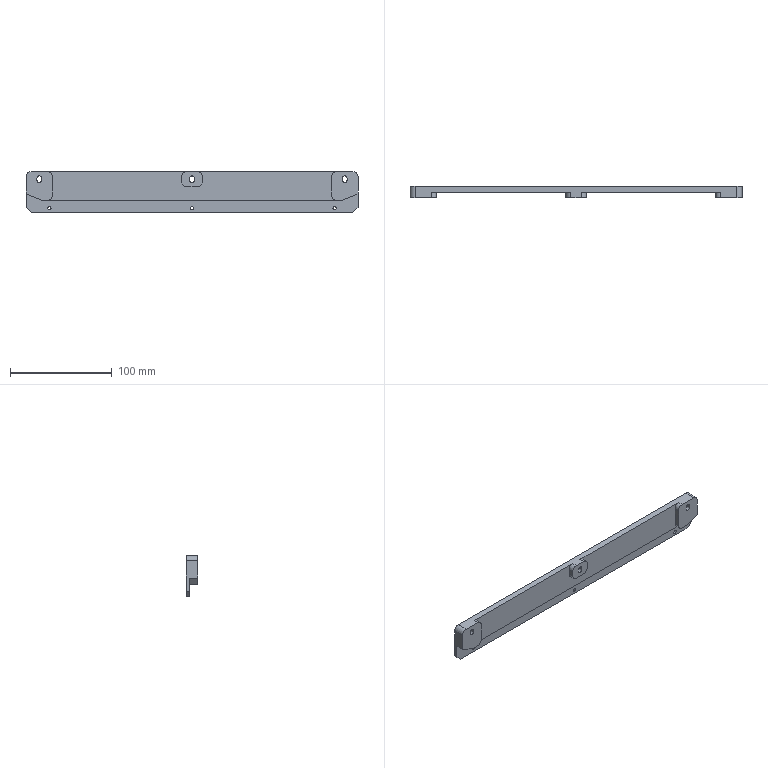Part | STEP file | upper limit plate 2 | 1 solid | 69 faces | box 326 x 11 x 40 mm | volume 72637 mm3 | plane 35 | cylinder 34 | commonest cylinder face diameters 10 x10 4.5 x9 8 x9 3.3 x6